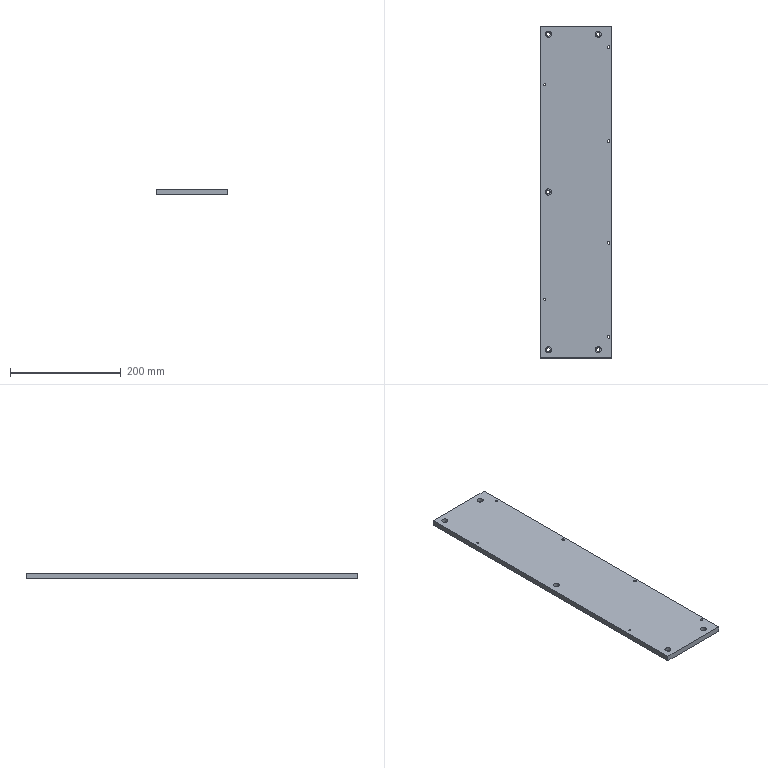Part | SolidWorks | features HoleWzd 3, Extrusion 1 | 1 solid | 55 faces | box 130 x 600 x 10 mm | volume 774782 mm3 | cylinder 40 | plane 15 | commonest cylinder face diameters 6.6 x10 11 x10 4.5 x8 8 x8 3.3 x4